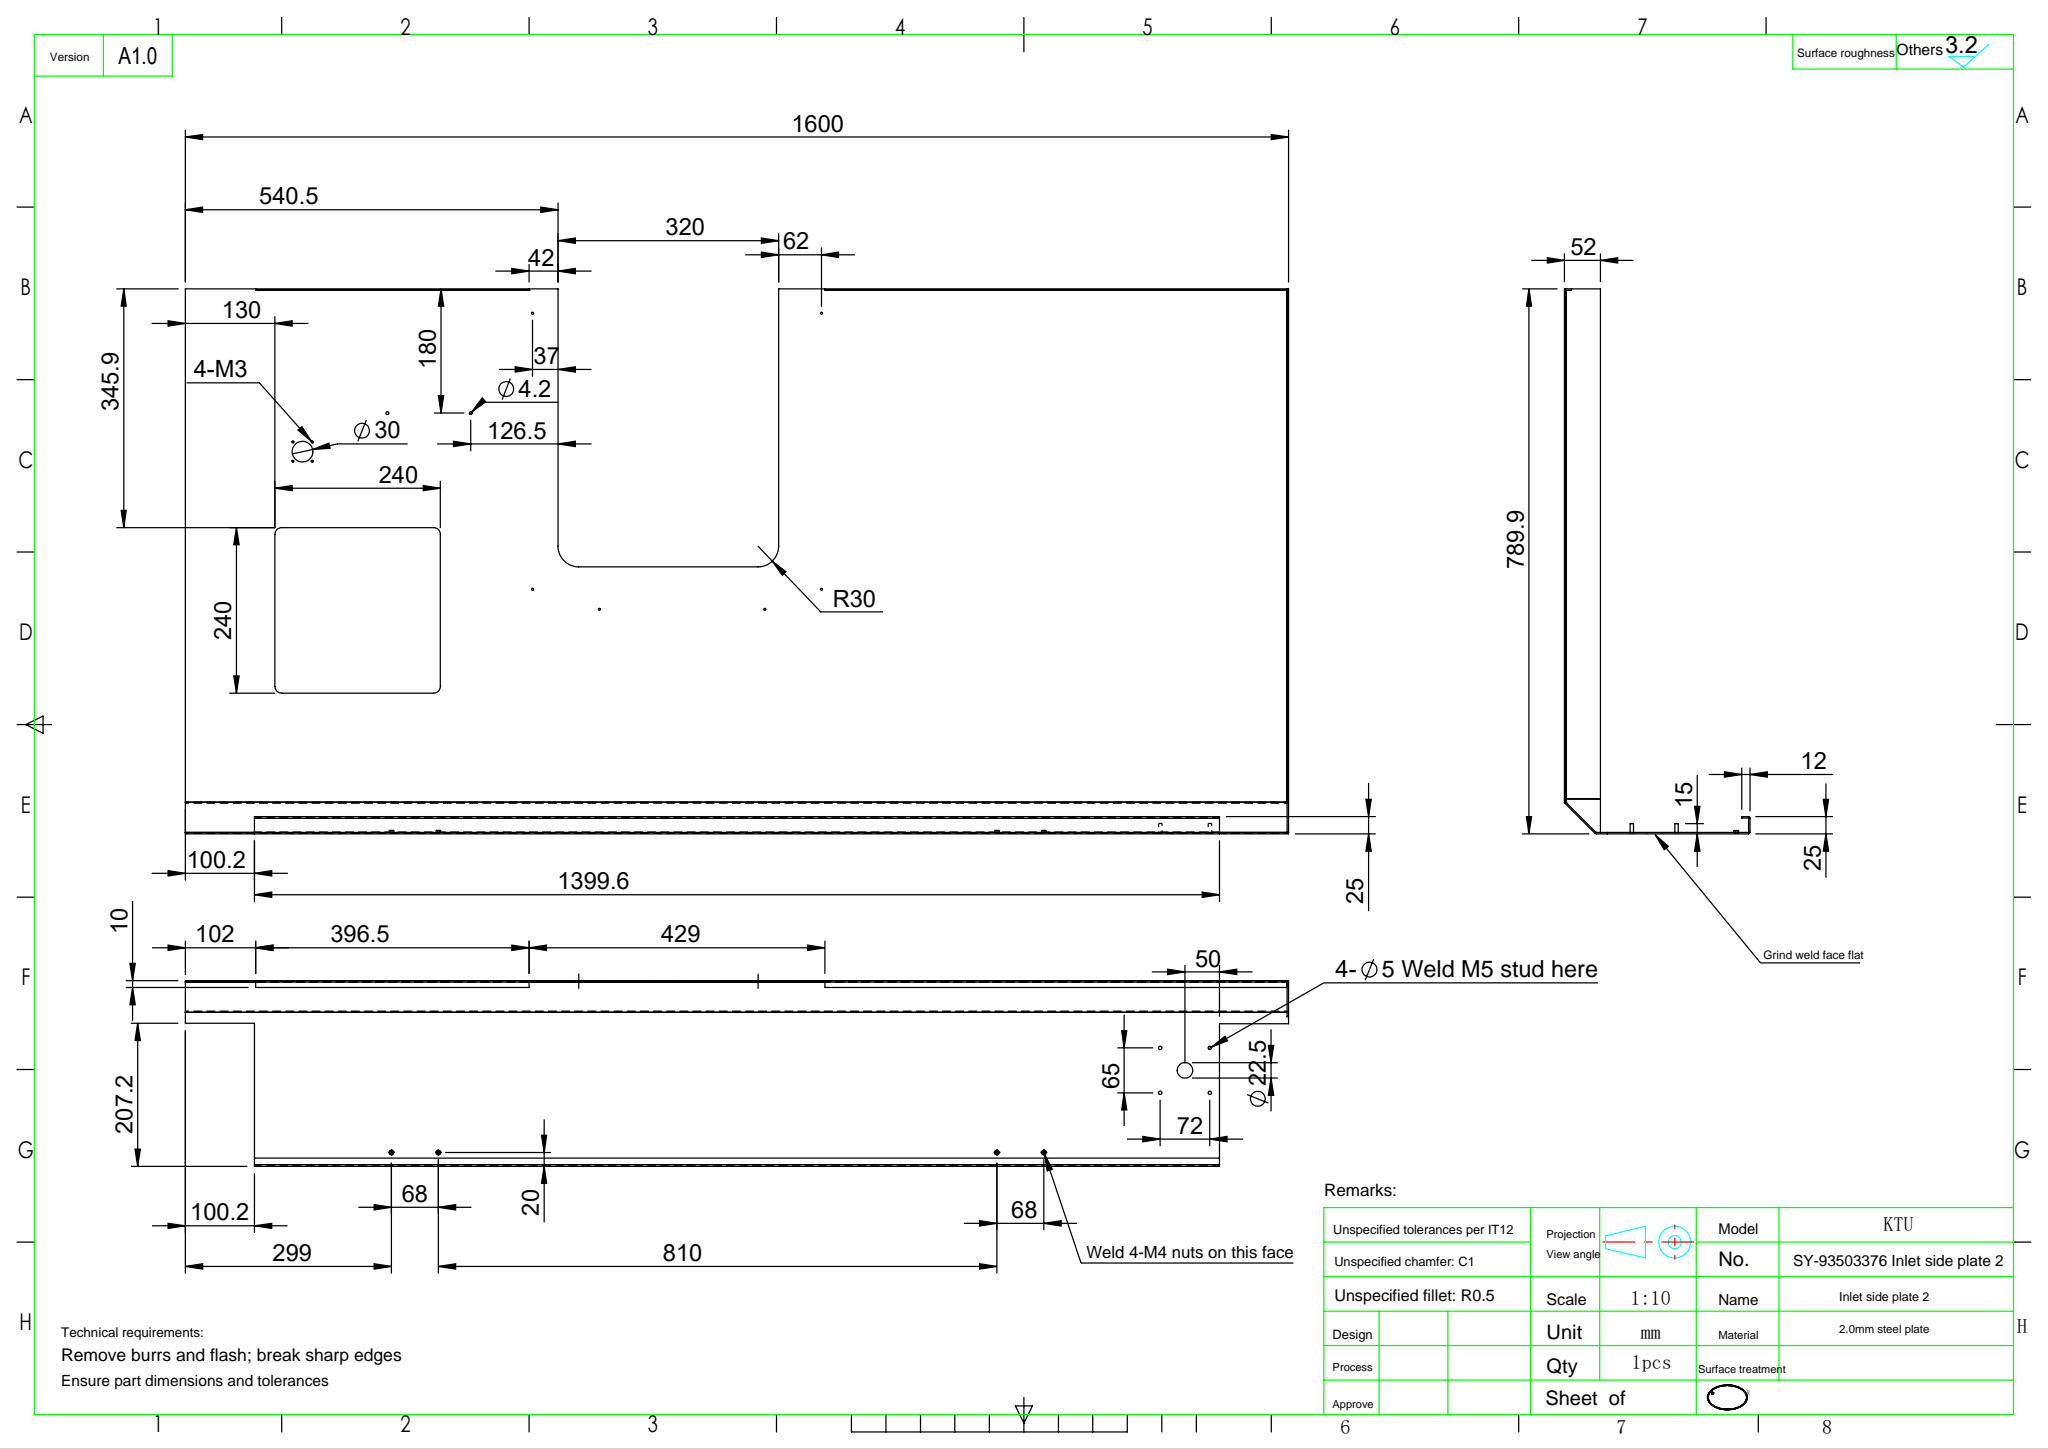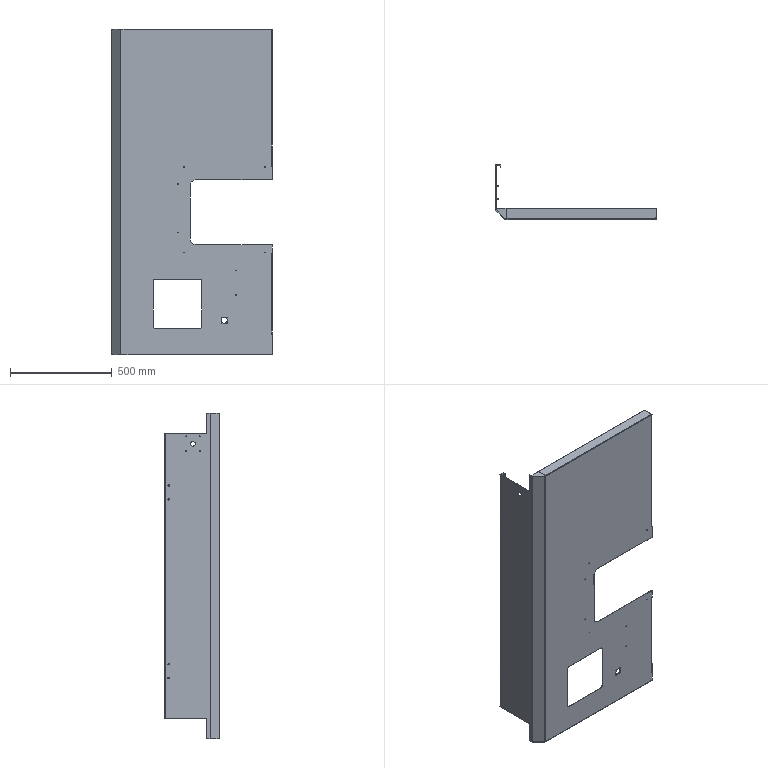Part | SolidWorks | features ICE 12, EdgeFlange 4, HoleWzd 4, Cut 3, 3DProfileFeature 2, FlatPattern 2, SMBaseFlange 2, SheetMetal 2, DelFace 1 | 6 solids | 174 faces | box 789.9 x 269 x 1600 mm | volume 3023926 mm3 | plane 92 | cylinder 82 | commonest cylinder face diameters 5 x16 3 x12 4.4 x9 2.5 x8 3.3 x8 7 x8